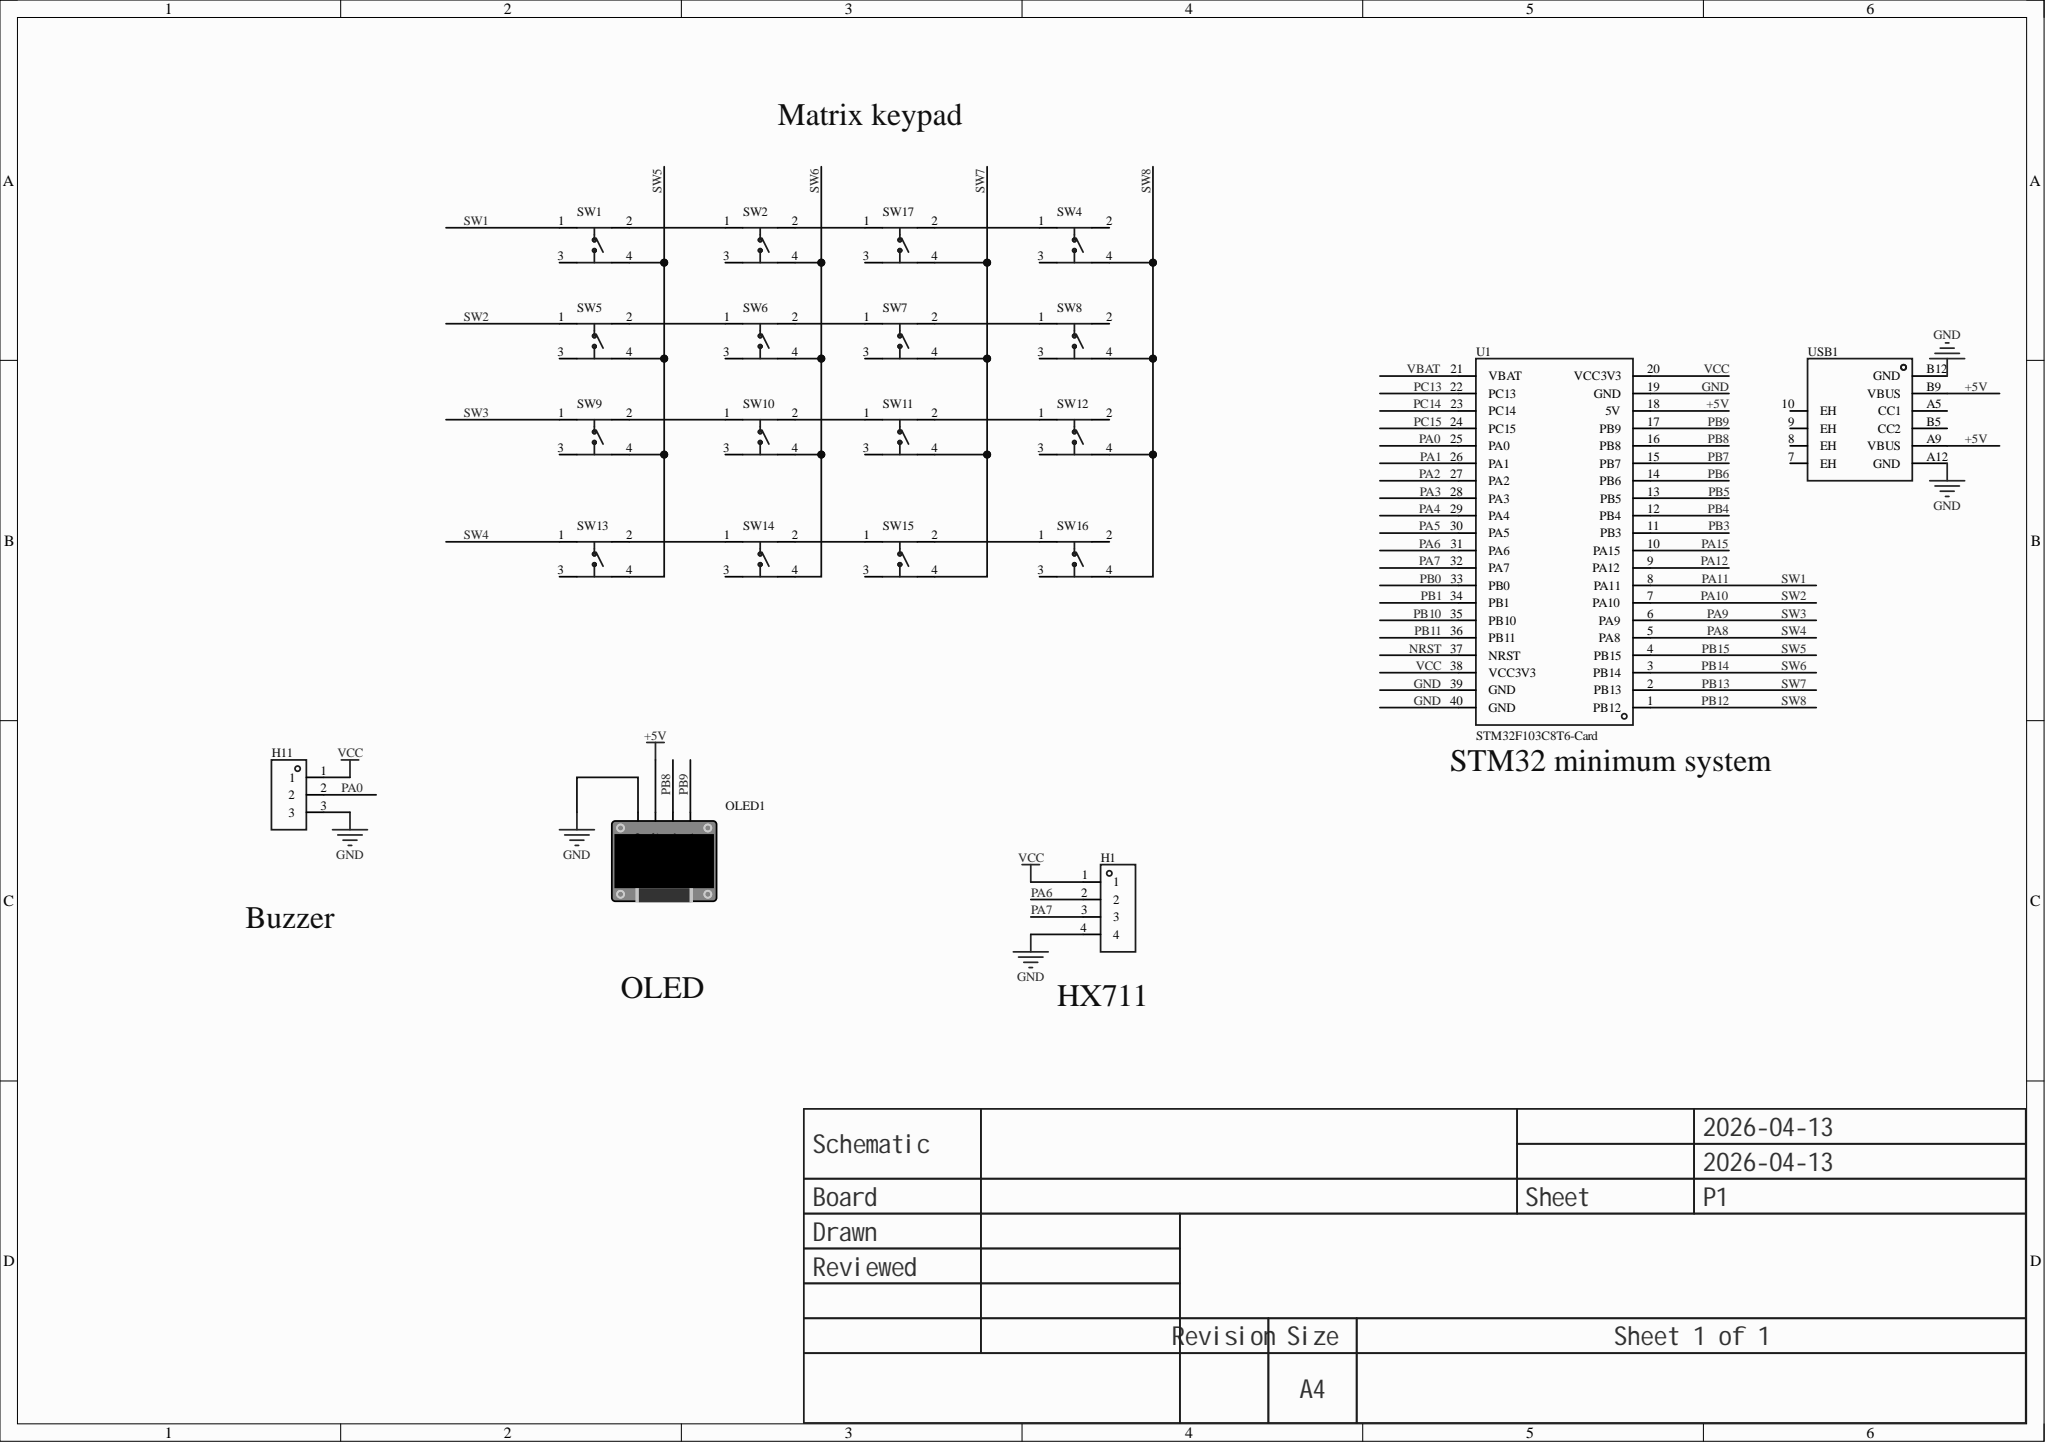Circuit board | Altium Designer | 21 parts | 28 nets
Bill of materials:
Comment,Description,Designator,Footprint,LibRef,Quantity
"","","H1","HDR-TH_4P-P2.54-V-M","HDR-M_2.54_1x4P","1"
"","","H11","HDR-TH_3P-P2.54-V-F","HDR-F_2.54_1x3P","1"
"","","OLED1","0.96OLED_4P","0.96OLED模块_4P","1"
"KH-6X6X6H-TJ","Circuit structure: SPST; Button shape: round button; Actuating force: 2.6N; Mounting: through-hole; Switch length: 6mm; Switch width: 6mm; Switch height: 6mm; Bracket: none; Contact current: 50mA; Rated voltage: 12V; Operating life: -;","SW1, SW2, SW4, SW5, SW6, SW7, SW8, SW9, SW10, SW11, SW12, SW13, SW14, SW15, SW16, SW17","SW-TH_4P-L6.0-W6.0-P4.50-LS6.5","KH-6X6X6H-TJ","16"
"STM32F103C8T6-Card","","U1","CONN-TH_L53.3-W22.9_STM32F103C8T6-CARD","STM32F103C8T6-Card","1"
"","","USB1","USB_ TYPE-C-6P","USB_ Type-C-6P","1"
Netlist (Protel format):
[
H1
HDR-TH_4P-P2.54-V-M




]
[
H11
HDR-TH_3P-P2.54-V-F




]
[
OLED1
0.96OLED_4P




]
[
SW1
SW-TH_4P-L6.0-W6.0-P4.50-LS6.5
KH-6X6X6H-TJ



]
[
SW2
SW-TH_4P-L6.0-W6.0-P4.50-LS6.5
KH-6X6X6H-TJ



]
[
SW4
SW-TH_4P-L6.0-W6.0-P4.50-LS6.5
KH-6X6X6H-TJ



]
[
SW5
SW-TH_4P-L6.0-W6.0-P4.50-LS6.5
KH-6X6X6H-TJ



]
[
SW6
SW-TH_4P-L6.0-W6.0-P4.50-LS6.5
KH-6X6X6H-TJ



]
[
SW7
SW-TH_4P-L6.0-W6.0-P4.50-LS6.5
KH-6X6X6H-TJ



]
[
SW8
SW-TH_4P-L6.0-W6.0-P4.50-LS6.5
KH-6X6X6H-TJ



]
[
SW9
SW-TH_4P-L6.0-W6.0-P4.50-LS6.5
KH-6X6X6H-TJ



]
[
SW10
SW-TH_4P-L6.0-W6.0-P4.50-LS6.5
KH-6X6X6H-TJ



]
[
SW11
SW-TH_4P-L6.0-W6.0-P4.50-LS6.5
KH-6X6X6H-TJ



]
[
SW12
SW-TH_4P-L6.0-W6.0-P4.50-LS6.5
KH-6X6X6H-TJ



]
[
SW13
SW-TH_4P-L6.0-W6.0-P4.50-LS6.5
KH-6X6X6H-TJ



]
[
SW14
SW-TH_4P-L6.0-W6.0-P4.50-LS6.5
KH-6X6X6H-TJ



]
[
SW15
SW-TH_4P-L6.0-W6.0-P4.50-LS6.5
KH-6X6X6H-TJ



]
[
SW16
SW-TH_4P-L6.0-W6.0-P4.50-LS6.5
KH-6X6X6H-TJ



]
[
SW17
SW-TH_4P-L6.0-W6.0-P4.50-LS6.5
KH-6X6X6H-TJ



]
[
U1
CONN-TH_L53.3-W22.9_STM32F103C8T6-CARD
STM32F103C8T6-Card



]
[
USB1
USB_ TYPE-C-6P




]
(
VCC
H1-1
H11-1
U1-20
U1-38
)
(
PB15
SW1-4
SW5-4
SW9-4
SW13-4
U1-4
)
(
PB14
SW2-4
SW6-4
SW10-4
SW14-4
U1-3
)
(
PB13
SW7-4
SW11-4
SW15-4
SW17-4
U1-2
)
(
PB12
SW4-4
SW8-4
SW12-4
SW16-4
U1-1
)
(
PB9
OLED1-4
U1-17
)
(
PB8
OLED1-3
U1-16
)
(
PA11
SW1-1
U1-8
)
(
PA10
SW5-1
U1-7
)
(
PA9
SW9-1
U1-6
)
(
PA8
SW13-1
U1-5
)
(
PA7
H1-3
U1-32
)
(
PA6
H1-2
U1-31
)
(
PA0
H11-2
U1-25
)
(
NetSW15_2
SW15-2
SW16-1
)
(
NetSW14_2
SW14-2
SW15-1
)
(
NetSW13_2
SW13-2
SW14-1
)
(
NetSW11_2
SW11-2
SW12-1
)
(
NetSW10_2
SW10-2
SW11-1
)
(
NetSW9_2
SW9-2
SW10-1
)
(
NetSW7_2
SW7-2
SW8-1
)
(
NetSW6_2
SW6-2
SW7-1
)
(
NetSW5_2
SW5-2
SW6-1
)
(
NetSW4_1
SW4-1
SW17-2
)
(
NetSW2_2
SW2-2
SW17-1
)
(
NetSW1_2
SW1-2
SW2-1
)
(
GND
H1-4
H11-3
OLED1-1
U1-19
U1-39
U1-40
USB1-A12
USB1-B12
)
(
+5V
OLED1-2
U1-18
USB1-A9
USB1-B9
)